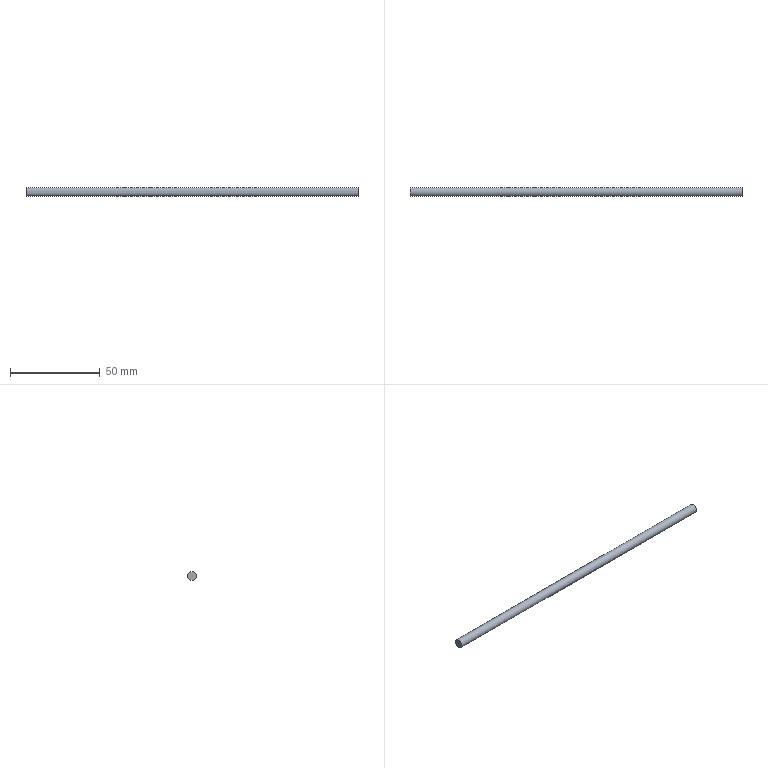Part | NX | features solid 2 | 1 solid | 3 faces | box 185 x 5 x 5 mm | volume 3632 mm3 | plane 2 | cylinder 1 | commonest cylinder face diameters 5 x1
STEP:
#1=CARTESIAN_POINT('',(-490.,377.5,-392.5));
#2=VERTEX_POINT('',#1);
#3=CARTESIAN_POINT('',(-490.,377.5,-395.));
#4=DIRECTION('',(-1.,0.,0.));
#5=DIRECTION('',(0.,0.,1.));
#6=AXIS2_PLACEMENT_3D('',#3,#4,#5);
#7=CIRCLE('',#6,2.5);
#8=EDGE_CURVE('',#2,#2,#7,.T.);
#9=ORIENTED_EDGE('',*,*,#8,.F.);
#10=EDGE_LOOP('',(#9));
#11=FACE_BOUND('',#10,.T.);
#12=CARTESIAN_POINT('',(-305.,377.5,-392.5));
#13=VERTEX_POINT('',#12);
#14=CARTESIAN_POINT('',(-305.,377.5,-395.));
#15=DIRECTION('',(-1.,0.,0.));
#16=DIRECTION('',(0.,0.,1.));
#17=AXIS2_PLACEMENT_3D('',#14,#15,#16);
#18=CIRCLE('',#17,2.5);
#19=EDGE_CURVE('',#13,#13,#18,.T.);
#20=ORIENTED_EDGE('',*,*,#19,.T.);
#21=EDGE_LOOP('',(#20));
#22=FACE_BOUND('',#21,.T.);
#23=CARTESIAN_POINT('',(-450.,377.5,-395.));
#24=DIRECTION('',(1.,0.,0.));
#25=DIRECTION('',(0.,0.,-1.));
#26=AXIS2_PLACEMENT_3D('',#23,#24,#25);
#27=CYLINDRICAL_SURFACE('',#26,2.5);
#28=ADVANCED_FACE('',(#11,#22),#27,.T.);
#29=ORIENTED_EDGE('',*,*,#8,.T.);
#30=EDGE_LOOP('',(#29));
#31=FACE_BOUND('',#30,.T.);
#32=CARTESIAN_POINT('',(-490.,377.5,-395.));
#33=DIRECTION('',(-1.,0.,0.));
#34=DIRECTION('',(0.,0.,1.));
#35=AXIS2_PLACEMENT_3D('',#32,#33,#34);
#36=PLANE('',#35);
#37=ADVANCED_FACE('',(#31),#36,.T.);
#38=ORIENTED_EDGE('',*,*,#19,.F.);
#39=EDGE_LOOP('',(#38));
#40=FACE_BOUND('',#39,.T.);
#41=CARTESIAN_POINT('',(-305.,377.5,-395.));
#42=DIRECTION('',(-1.,0.,0.));
#43=DIRECTION('',(0.,0.,1.));
#44=AXIS2_PLACEMENT_3D('',#41,#42,#43);
#45=PLANE('',#44);
#46=ADVANCED_FACE('',(#40),#45,.F.);
#47=CLOSED_SHELL('',(#28,#37,#46));
#48=MANIFOLD_SOLID_BREP('',#47);
#49=(LENGTH_UNIT()NAMED_UNIT(*)SI_UNIT(.MILLI.,.METRE.));
#50=UNCERTAINTY_MEASURE_WITH_UNIT(LENGTH_MEASURE(0.00001),#49,'','');
#51=(NAMED_UNIT(*)PLANE_ANGLE_UNIT()SI_UNIT($,.RADIAN.));
#52=(NAMED_UNIT(*)SI_UNIT($,.STERADIAN.)SOLID_ANGLE_UNIT());
#53=(GEOMETRIC_REPRESENTATION_CONTEXT(3)GLOBAL_UNCERTAINTY_ASSIGNED_CONTEXT((#50))GLOBAL_UNIT_ASSIGNED_CONTEXT((#49,#51,#52))REPRESENTATION_CONTEXT('',''));
#54=ADVANCED_BREP_SHAPE_REPRESENTATION('',(#48),#53);